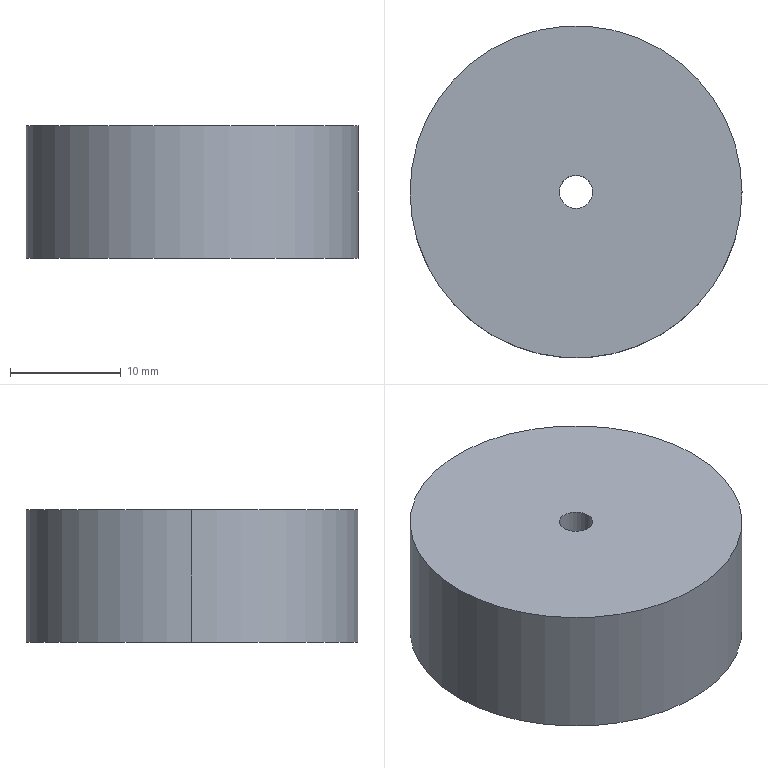Part | SolidWorks | features Extrusion 1 | 1 solid | 6 faces | box 30 x 30 x 12 mm | volume 8397 mm3 | cylinder 4 | plane 2 | commonest cylinder face diameters 3 x2 30 x2
STEP:
#1=CARTESIAN_POINT('',(-1.5,0.,12.));
#2=VERTEX_POINT('',#1);
#3=CARTESIAN_POINT('',(1.5,0.,12.));
#4=VERTEX_POINT('',#3);
#5=CARTESIAN_POINT('',(0.,0.,12.));
#6=DIRECTION('',(0.,0.,1.));
#7=DIRECTION('',(1.,0.,0.));
#8=AXIS2_PLACEMENT_3D('',#5,#6,#7);
#9=CIRCLE('',#8,1.5);
#10=EDGE_CURVE('',#2,#4,#9,.T.);
#11=ORIENTED_EDGE('',*,*,#10,.T.);
#12=CARTESIAN_POINT('',(1.5,0.,0.));
#13=VERTEX_POINT('',#12);
#14=CARTESIAN_POINT('',(1.5,0.,12.));
#15=DIRECTION('',(0.,0.,-1.));
#16=VECTOR('',#15,1000.);
#17=LINE('',#14,#16);
#18=EDGE_CURVE('',#4,#13,#17,.T.);
#19=ORIENTED_EDGE('',*,*,#18,.T.);
#20=CARTESIAN_POINT('',(-1.5,0.,0.));
#21=VERTEX_POINT('',#20);
#22=CARTESIAN_POINT('',(0.,0.,0.));
#23=DIRECTION('',(0.,0.,1.));
#24=DIRECTION('',(1.,0.,0.));
#25=AXIS2_PLACEMENT_3D('',#22,#23,#24);
#26=CIRCLE('',#25,1.5);
#27=EDGE_CURVE('',#21,#13,#26,.T.);
#28=ORIENTED_EDGE('',*,*,#27,.F.);
#29=CARTESIAN_POINT('',(-1.5,0.,12.));
#30=DIRECTION('',(0.,0.,-1.));
#31=VECTOR('',#30,1000.);
#32=LINE('',#29,#31);
#33=EDGE_CURVE('',#2,#21,#32,.T.);
#34=ORIENTED_EDGE('',*,*,#33,.F.);
#35=EDGE_LOOP('',(#11,#19,#28,#34));
#36=FACE_OUTER_BOUND('',#35,.T.);
#37=CARTESIAN_POINT('',(0.,0.,12.));
#38=DIRECTION('',(0.,0.,-1.));
#39=DIRECTION('',(-1.,0.,0.));
#40=AXIS2_PLACEMENT_3D('',#37,#38,#39);
#41=CYLINDRICAL_SURFACE('',#40,1.5);
#42=ADVANCED_FACE('',(#36),#41,.F.);
#43=CARTESIAN_POINT('',(15.,0.,12.));
#44=VERTEX_POINT('',#43);
#45=CARTESIAN_POINT('',(-15.,0.,12.));
#46=VERTEX_POINT('',#45);
#47=CARTESIAN_POINT('',(0.,0.,12.));
#48=DIRECTION('',(0.,0.,1.));
#49=DIRECTION('',(1.,0.,0.));
#50=AXIS2_PLACEMENT_3D('',#47,#48,#49);
#51=CIRCLE('',#50,15.);
#52=EDGE_CURVE('',#44,#46,#51,.T.);
#53=ORIENTED_EDGE('',*,*,#52,.F.);
#54=CARTESIAN_POINT('',(15.,0.,0.));
#55=VERTEX_POINT('',#54);
#56=CARTESIAN_POINT('',(15.,0.,12.));
#57=DIRECTION('',(0.,0.,-1.));
#58=VECTOR('',#57,1000.);
#59=LINE('',#56,#58);
#60=EDGE_CURVE('',#44,#55,#59,.T.);
#61=ORIENTED_EDGE('',*,*,#60,.T.);
#62=CARTESIAN_POINT('',(-15.,0.,0.));
#63=VERTEX_POINT('',#62);
#64=CARTESIAN_POINT('',(0.,0.,0.));
#65=DIRECTION('',(0.,0.,1.));
#66=DIRECTION('',(1.,0.,0.));
#67=AXIS2_PLACEMENT_3D('',#64,#65,#66);
#68=CIRCLE('',#67,15.);
#69=EDGE_CURVE('',#55,#63,#68,.T.);
#70=ORIENTED_EDGE('',*,*,#69,.T.);
#71=CARTESIAN_POINT('',(-15.,0.,12.));
#72=DIRECTION('',(0.,0.,-1.));
#73=VECTOR('',#72,1000.);
#74=LINE('',#71,#73);
#75=EDGE_CURVE('',#46,#63,#74,.T.);
#76=ORIENTED_EDGE('',*,*,#75,.F.);
#77=EDGE_LOOP('',(#53,#61,#70,#76));
#78=FACE_OUTER_BOUND('',#77,.T.);
#79=CARTESIAN_POINT('',(0.,0.,12.));
#80=DIRECTION('',(0.,0.,-1.));
#81=DIRECTION('',(-1.,0.,0.));
#82=AXIS2_PLACEMENT_3D('',#79,#80,#81);
#83=CYLINDRICAL_SURFACE('',#82,15.);
#84=ADVANCED_FACE('',(#78),#83,.T.);
#85=CARTESIAN_POINT('',(0.,0.,12.));
#86=DIRECTION('',(0.,0.,1.));
#87=DIRECTION('',(1.,0.,0.));
#88=AXIS2_PLACEMENT_3D('',#85,#86,#87);
#89=CIRCLE('',#88,15.);
#90=EDGE_CURVE('',#46,#44,#89,.T.);
#91=ORIENTED_EDGE('',*,*,#90,.T.);
#92=ORIENTED_EDGE('',*,*,#52,.T.);
#93=EDGE_LOOP('',(#91,#92));
#94=FACE_OUTER_BOUND('',#93,.T.);
#95=ORIENTED_EDGE('',*,*,#10,.F.);
#96=CARTESIAN_POINT('',(0.,0.,12.));
#97=DIRECTION('',(0.,0.,1.));
#98=DIRECTION('',(1.,0.,0.));
#99=AXIS2_PLACEMENT_3D('',#96,#97,#98);
#100=CIRCLE('',#99,1.5);
#101=EDGE_CURVE('',#4,#2,#100,.T.);
#102=ORIENTED_EDGE('',*,*,#101,.F.);
#103=EDGE_LOOP('',(#95,#102));
#104=FACE_BOUND('',#103,.T.);
#105=CARTESIAN_POINT('',(0.,0.,12.));
#106=DIRECTION('',(0.,0.,1.));
#107=DIRECTION('',(1.,0.,0.));
#108=AXIS2_PLACEMENT_3D('',#105,#106,#107);
#109=PLANE('',#108);
#110=ADVANCED_FACE('',(#94,#104),#109,.T.);
#111=CARTESIAN_POINT('',(0.,0.,0.));
#112=DIRECTION('',(0.,0.,1.));
#113=DIRECTION('',(1.,0.,0.));
#114=AXIS2_PLACEMENT_3D('',#111,#112,#113);
#115=CIRCLE('',#114,15.);
#116=EDGE_CURVE('',#63,#55,#115,.T.);
#117=ORIENTED_EDGE('',*,*,#116,.F.);
#118=ORIENTED_EDGE('',*,*,#69,.F.);
#119=EDGE_LOOP('',(#117,#118));
#120=FACE_OUTER_BOUND('',#119,.T.);
#121=ORIENTED_EDGE('',*,*,#27,.T.);
#122=CARTESIAN_POINT('',(0.,0.,0.));
#123=DIRECTION('',(0.,0.,1.));
#124=DIRECTION('',(1.,0.,0.));
#125=AXIS2_PLACEMENT_3D('',#122,#123,#124);
#126=CIRCLE('',#125,1.5);
#127=EDGE_CURVE('',#13,#21,#126,.T.);
#128=ORIENTED_EDGE('',*,*,#127,.T.);
#129=EDGE_LOOP('',(#121,#128));
#130=FACE_BOUND('',#129,.T.);
#131=CARTESIAN_POINT('',(0.,0.,0.));
#132=DIRECTION('',(0.,0.,1.));
#133=DIRECTION('',(1.,0.,0.));
#134=AXIS2_PLACEMENT_3D('',#131,#132,#133);
#135=PLANE('',#134);
#136=ADVANCED_FACE('',(#120,#130),#135,.F.);
#137=ORIENTED_EDGE('',*,*,#60,.F.);
#138=ORIENTED_EDGE('',*,*,#90,.F.);
#139=ORIENTED_EDGE('',*,*,#75,.T.);
#140=ORIENTED_EDGE('',*,*,#116,.T.);
#141=EDGE_LOOP('',(#137,#138,#139,#140));
#142=FACE_OUTER_BOUND('',#141,.T.);
#143=CARTESIAN_POINT('',(0.,0.,12.));
#144=DIRECTION('',(0.,0.,-1.));
#145=DIRECTION('',(-1.,0.,0.));
#146=AXIS2_PLACEMENT_3D('',#143,#144,#145);
#147=CYLINDRICAL_SURFACE('',#146,15.);
#148=ADVANCED_FACE('',(#142),#147,.T.);
#149=ORIENTED_EDGE('',*,*,#18,.F.);
#150=ORIENTED_EDGE('',*,*,#101,.T.);
#151=ORIENTED_EDGE('',*,*,#33,.T.);
#152=ORIENTED_EDGE('',*,*,#127,.F.);
#153=EDGE_LOOP('',(#149,#150,#151,#152));
#154=FACE_OUTER_BOUND('',#153,.T.);
#155=CARTESIAN_POINT('',(0.,0.,12.));
#156=DIRECTION('',(0.,0.,-1.));
#157=DIRECTION('',(-1.,0.,0.));
#158=AXIS2_PLACEMENT_3D('',#155,#156,#157);
#159=CYLINDRICAL_SURFACE('',#158,1.5);
#160=ADVANCED_FACE('',(#154),#159,.F.);
#161=CLOSED_SHELL('',(#42,#84,#110,#136,#148,#160));
#162=MANIFOLD_SOLID_BREP('',#161);
#163=CARTESIAN_POINT('',(0.,0.,0.));
#164=DIRECTION('',(0.,0.,1.));
#165=DIRECTION('',(1.,0.,0.));
#166=AXIS2_PLACEMENT_3D('',#163,#164,#165);
#167=(LENGTH_UNIT()NAMED_UNIT(*)SI_UNIT(.MILLI.,.METRE.));
#168=UNCERTAINTY_MEASURE_WITH_UNIT(LENGTH_MEASURE(0.00001),#167,'','');
#169=(NAMED_UNIT(*)PLANE_ANGLE_UNIT()SI_UNIT($,.RADIAN.));
#170=(NAMED_UNIT(*)SI_UNIT($,.STERADIAN.)SOLID_ANGLE_UNIT());
#171=(GEOMETRIC_REPRESENTATION_CONTEXT(3)GLOBAL_UNCERTAINTY_ASSIGNED_CONTEXT((#168))GLOBAL_UNIT_ASSIGNED_CONTEXT((#167,#169,#170))REPRESENTATION_CONTEXT('',''));
#172=ADVANCED_BREP_SHAPE_REPRESENTATION('',(#162,#166),#171);